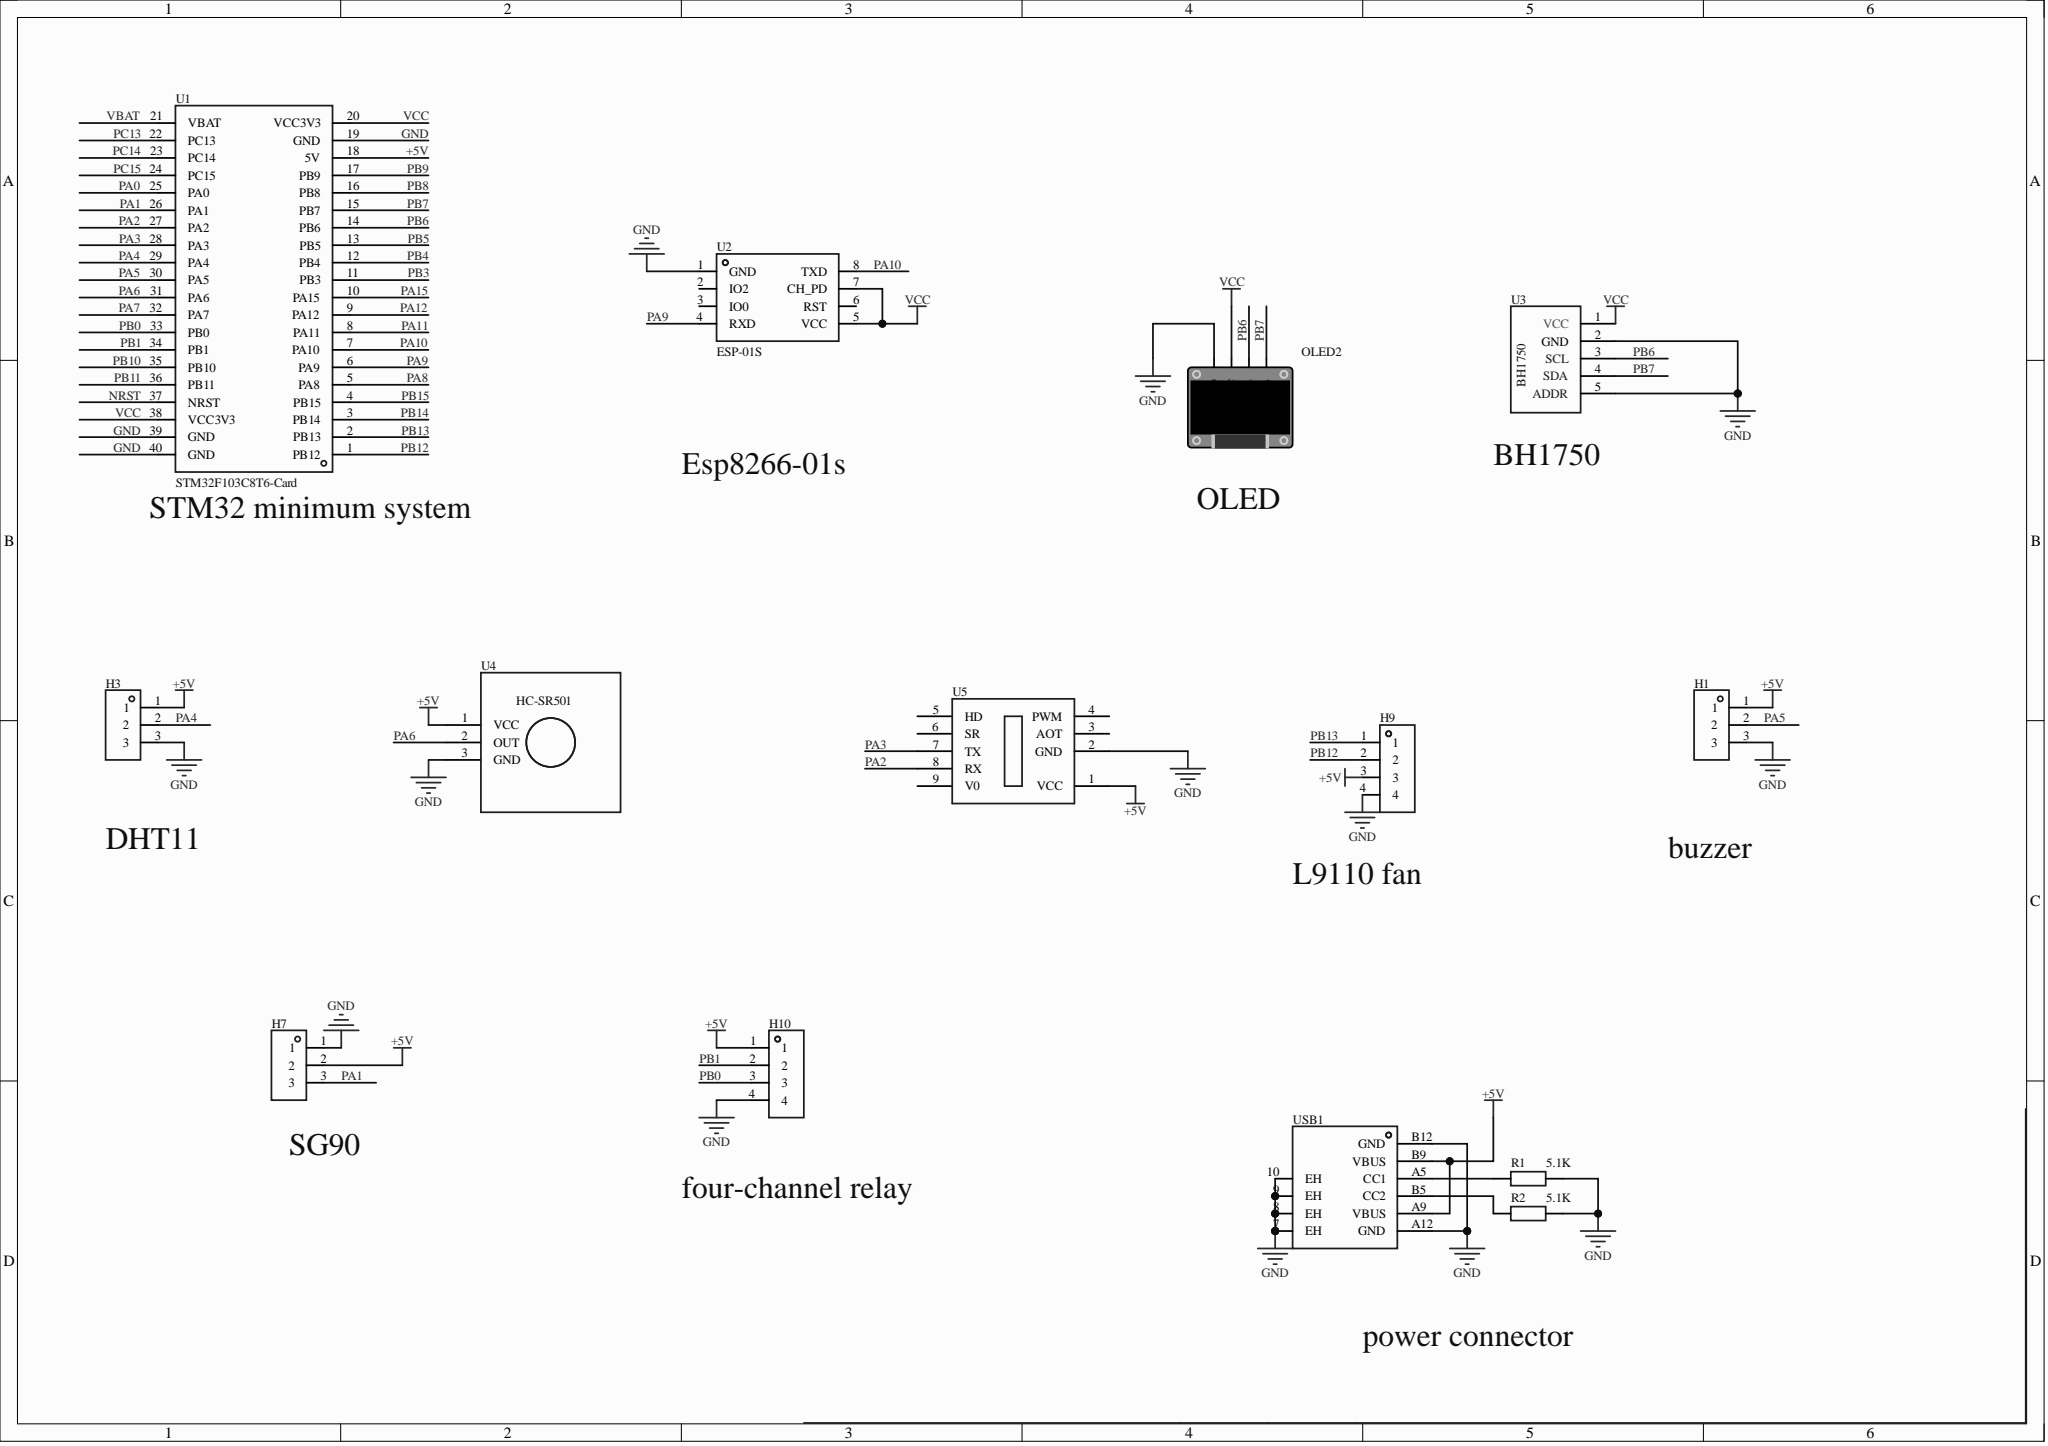Circuit board | Altium Designer | 14 parts | 19 nets
Bill of materials:
Comment,Description,Designator,Footprint,LibRef,Quantity
"","","H1, H3, H7","HDR-TH_3P-P2.54-V-F","HDR-F_2.54_1x3P","3"
"","","H9, H10","HDR-TH_4P-P2.54-V-F","HDR-F_2.54_1x4P","2"
"","","OLED2","0.96OLED_4P","0.96OLED模块_4P","1"
"5.1K","","R1, R2","R0805","Res_0805","2"
"STM32F103C8T6-Card","","U1","CONN-TH_L53.3-W22.9_STM32F103C8T6-CARD","STM32F103C8T6-Card","1"
"ESP-01S","","U2","WIFIM-TH_ESP-01S","ESP-01S_C111009","1"
"","","U3","BH1750光照传感器","BH1750光照传感器","1"
"","","U4","HC-SR501_W32_H24","HC-SR501","1"
"","","U5","MH-Z19C-9PIN","MH-Z19C","1"
"","","USB1","USB_ TYPE-C-6P","USB_ Type-C-6P","1"
Netlist (Protel format):
[
H1
HDR-TH_3P-P2.54-V-F




]
[
H3
HDR-TH_3P-P2.54-V-F




]
[
H7
HDR-TH_3P-P2.54-V-F




]
[
H9
HDR-TH_4P-P2.54-V-F




]
[
H10
HDR-TH_4P-P2.54-V-F




]
[
OLED2
0.96OLED_4P




]
[
R1
R0805
5.1K



]
[
R2
R0805
5.1K



]
[
U1
CONN-TH_L53.3-W22.9_STM32F103C8T6-CARD
STM32F103C8T6-Card



]
[
U2
WIFIM-TH_ESP-01S
ESP-01S



]
[
U3
BH1750光照传感器




]
[
U4
HC-SR501_W32_H24




]
[
U5
MH-Z19C-9PIN




]
[
USB1
USB_ TYPE-C-6P




]
(
VCC
OLED2-2
U1-20
U1-38
U2-5
U2-7
U3-1
)
(
PB13
H9-1
U1-2
)
(
PB12
H9-2
U1-1
)
(
PB7
OLED2-4
U1-15
U3-4
)
(
PB6
OLED2-3
U1-14
U3-3
)
(
PB1
H10-2
U1-34
)
(
PB0
H10-3
U1-33
)
(
PA10
U1-7
U2-8
)
(
PA9
U1-6
U2-4
)
(
PA6
U1-31
U4-2
)
(
PA5
H1-2
U1-30
)
(
PA4
H3-2
U1-29
)
(
PA3
U1-28
U5-7
)
(
PA2
U1-27
U5-8
)
(
PA1
H7-3
U1-26
)
(
NetR2_1
R2-1
USB1-B5
)
(
NetR1_1
R1-1
USB1-A5
)
(
GND
H1-3
H3-3
H7-1
H9-4
H10-4
OLED2-1
R1-2
R2-2
U1-19
U1-39
U1-40
U2-1
U3-2
U3-5
U4-3
U5-2
USB1-7
USB1-8
USB1-9
USB1-10
USB1-A12
USB1-B12
)
(
+5V
H1-1
H3-1
H7-2
H9-3
H10-1
U1-18
U4-1
U5-1
USB1-A9
USB1-B9
)